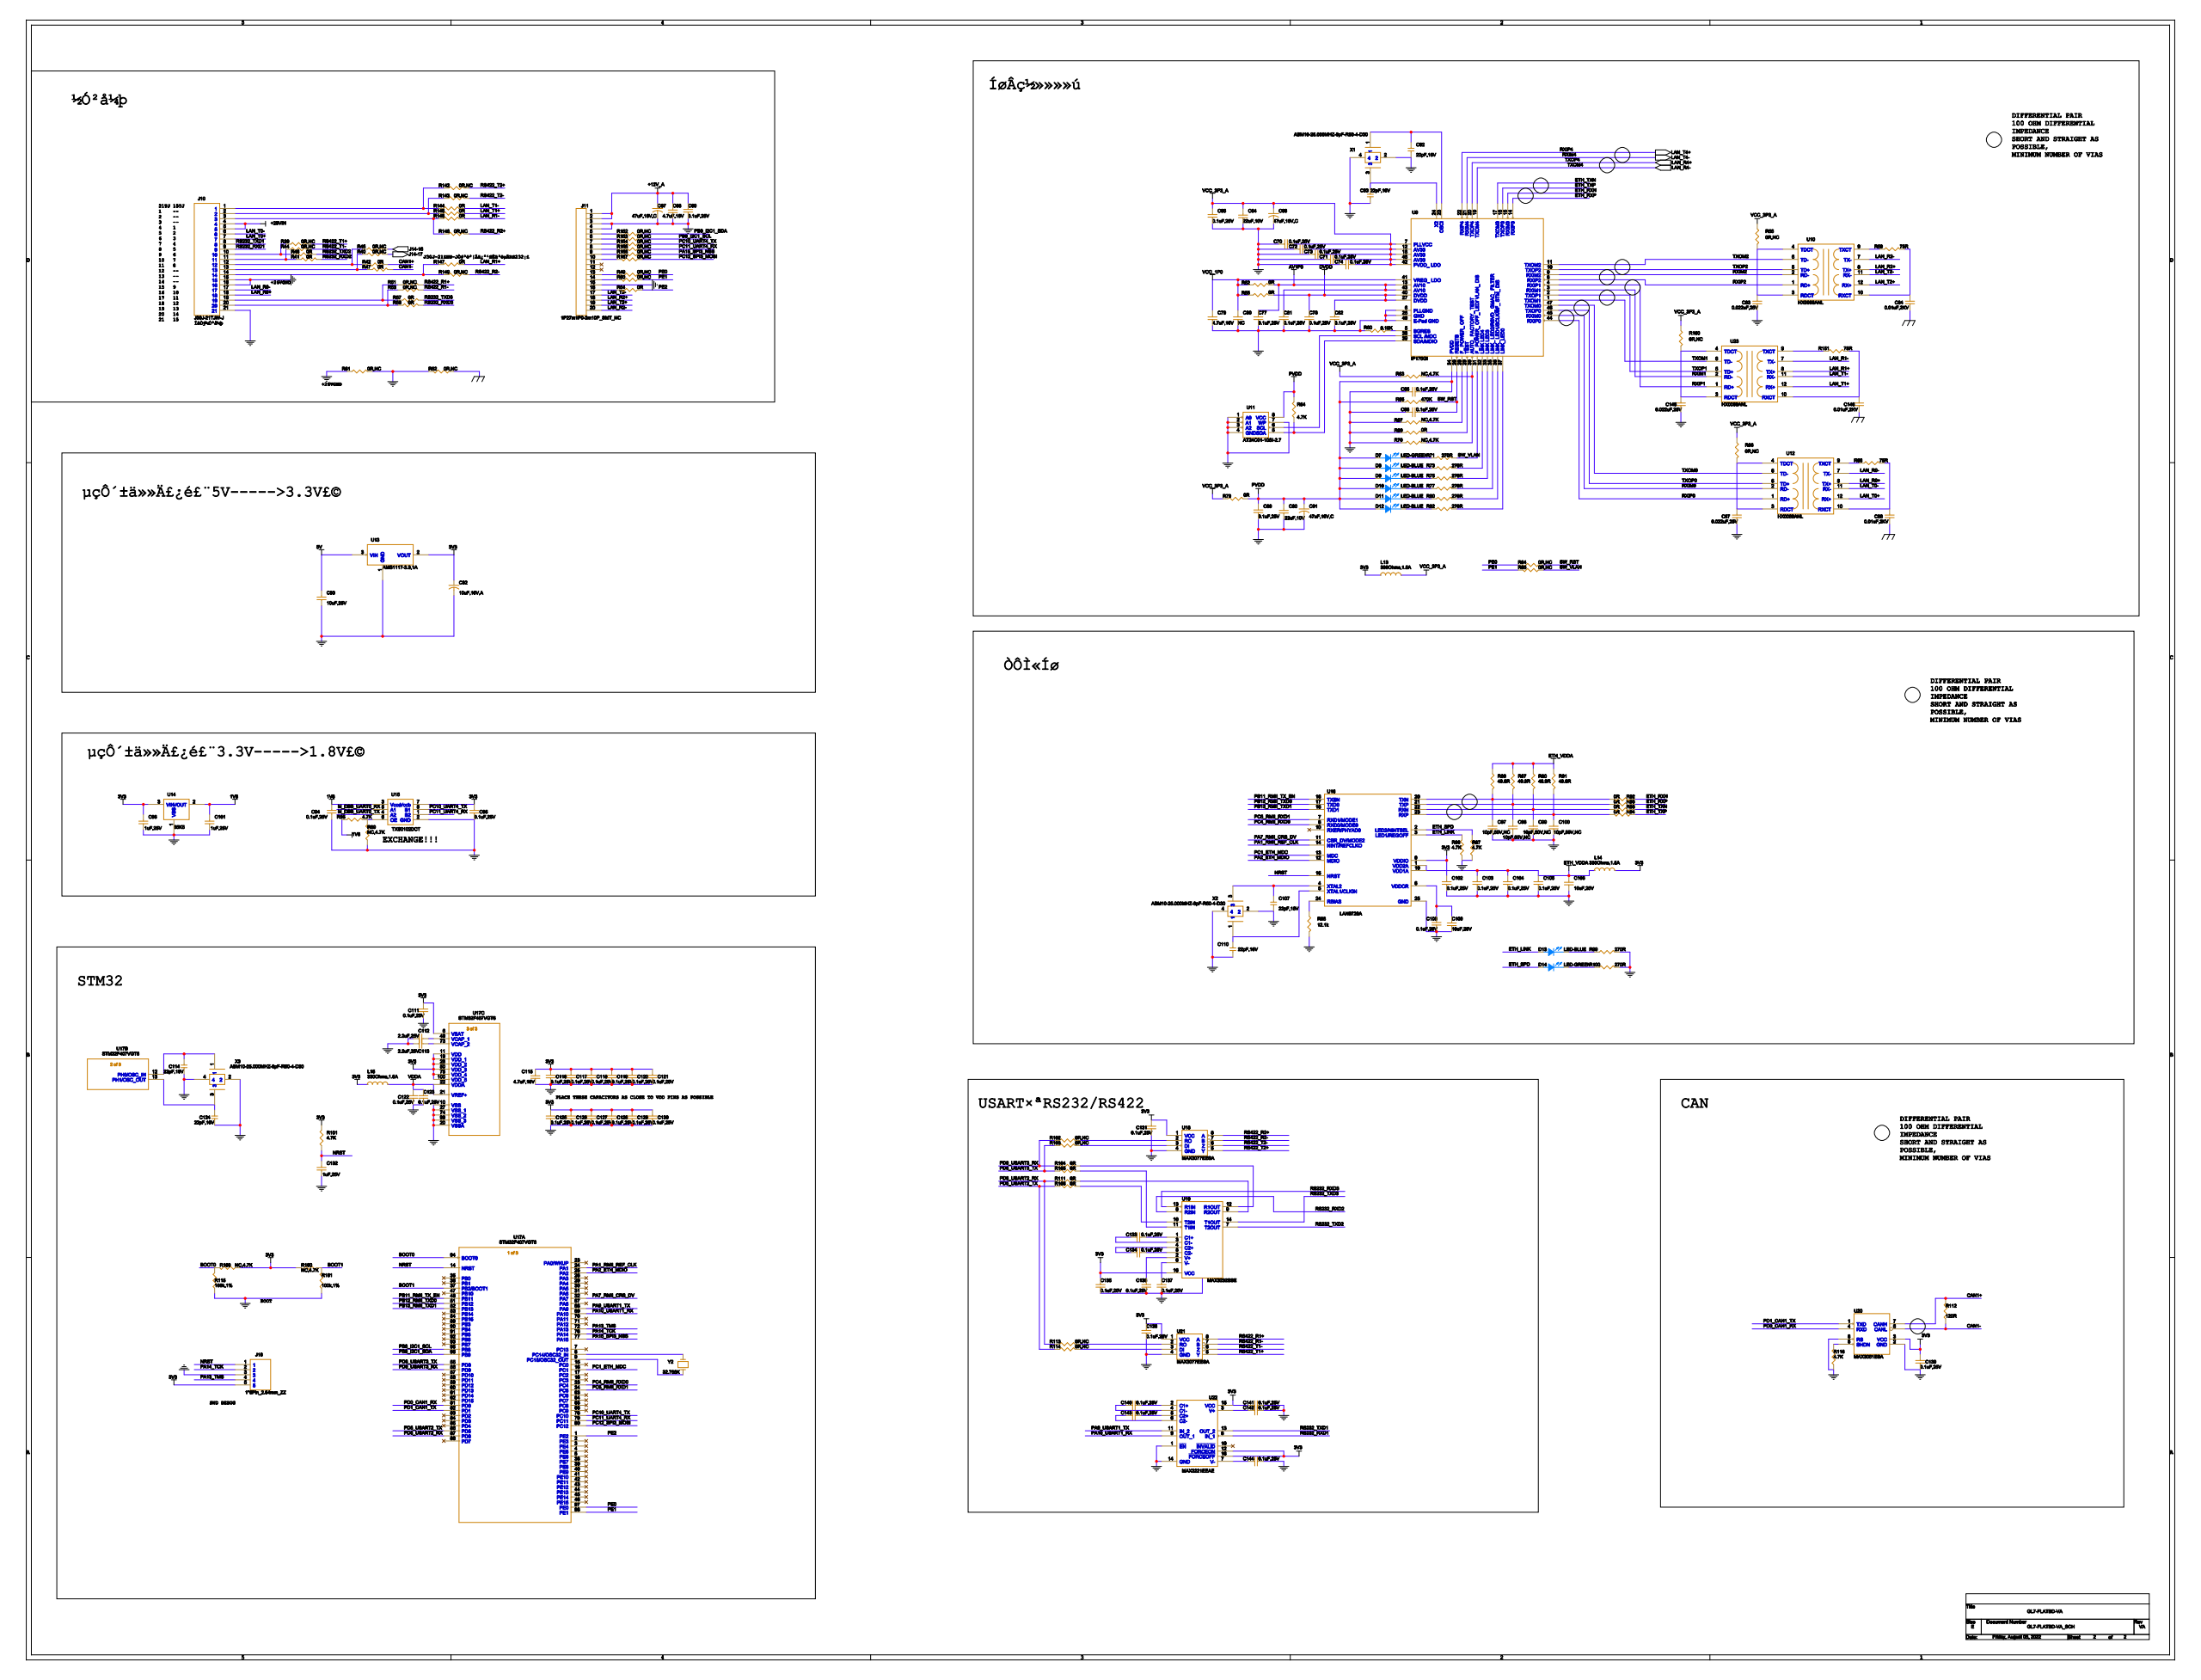Circuit board | Cadence Allegro | 338 parts | 273 nets | one sheet of the schematic
Parts on this sheet (reference | value | footprint):
C62 | 22pF,16V | 0402C
C63 | 22pF,16V | 0402C
C64 | 22uF,10V | 0603C
C65 | 0.1uF,25V | 0201C
C66 | 47uF,16V,C | CA45C
C67 | 47uF,16V,C | CA45C
C68 | 4.7uF,16V | 0603C
C69 | 0.1uF,25V | 0201C
C70 | 0.1uF,25V | 0201C
C71 | 0.1uF,25V | 0201C
C72 | 0.1uF,25V | 0201C
C73 | 0.1uF,25V | 0201C
C74 | 0.1uF,25V | 0201C
C77 | 0.1uF,25V | 0201C
C78 | 0.1uF,25V | 0201C
C79 | 4.7uF,16V | 0603C
C80 | NC | 0402C
C81 | 0.1uF,25V | 0201C
C82 | 0.1uF,25V | 0201C
C83 | 0.022uF,25V | 0402C
C84 | 0.01uF,2KV | 1812C
C85 | 0.1uF,25V | 0201C
C86 | 0.1uF,25V | 0201C
C87 | 0.022uF,25V | 0402C
C88 | 0.01uF,2KV | 1812C
C89 | 0.1uF,25V | 0201C
C90 | 22uF,10V | 0603C
C91 | 47uF,16V,C | CA45C
C92 | 10uF,16V,A | CA45A
C93 | 10uF,25V | 1206C
C94 | 0.1uF,25V | 0201C
C95 | 0.1uF,25V | 0201C
C96 | 1uF,25V | 0402C
C97 | NC | 0402C
C98 | NC | 0402C
C99 | NC | 0402C
C100 | NC | 0402C
C101 | 1uF,25V | 0402C
C102 | 0.1uF,25V | 0201C
C103 | 0.1uF,25V | 0201C
C104 | 0.1uF,25V | 0201C
C105 | 0.1uF,25V | 0201C
C106 | 10uF,25V | 1206C
C107 | 22pF,16V | 0402C
C108 | 0.1uF,25V | 0201C
C109 | 10uF,25V | 1206C
C110 | 22pF,16V | 0402C
C111 | 0.1uF,25V | 0201C
C112 | 2.2uF,25V | 0603C
C114 | 22pF,16V | 0402C
C115 | 4.7uF,16V | 0603C
C116 | 0.1uF,25V | 0201C
C117 | 0.1uF,25V | 0201C
C118 | 0.1uF,25V | 0201C
C119 | 0.1uF,25V | 0201C
C120 | 0.1uF,25V | 0201C
C121 | 0.1uF,25V | 0201C
C122 | 0.1uF,25V | 0201C
C123 | 0.1uF,25V | 0201C
C124 | 22pF,16V | 0402C
C125 | 0.1uF,25V | 0201C
C126 | 0.1uF,25V | 0201C
C127 | 0.1uF,25V | 0201C
C128 | 0.1uF,25V | 0201C
C129 | 0.1uF,25V | 0201C
C130 | 0.1uF,25V | 0201C
C131 | 0.1uF,25V | 0201C
C132 | 1uF,25V | 0402C
C133 | 0.1uF,25V | 0201C
C134 | 0.1uF,25V | 0201C
C135 | 0.1uF,25V | 0201C
C136 | 0.1uF,25V | 0201C
C137 | 0.1uF,25V | 0201C
C138 | 0.1uF,25V | 0201C
C139 | 0.1uF,25V | 0201C
C140 | 0.1uF,25V | 0201C
C141 | 0.1uF,25V | 0201C
C142 | 0.1uF,25V | 0201C
C143 | 0.1uF,25V | 0201C
C144 | 0.1uF,25V | 0201C
C145 | 0.022uF,25V | 0402C
C146 | 0.01uF,2KV | 1812C
D7 | LED-GREEN | 0603L
D8 | LED-BLUE | 0603L
D9 | LED-BLUE | 0603L
D10 | LED-BLUE | 0603L
D11 | LED-BLUE | 0603L
D12 | LED-BLUE | 0603L
D13 | LED-BLUE | 0603L
D14 | LED-GREEN | 0603L
J10 | J30J-21TJW-J | J30J-21TJW-J
J11 | 1P27m1P0-2m10P_SMT_NC | 1P27-2-10-L-SMT
J16 | 1*5Pin_2.54mm_ZZ | SIP-5-2R5
L13 | 330Ohms,1.5A | 0805L
L14 | 1.5A,330Ohms | 0805L
L15 | 1.5A,330Ohms | 0805L
R39 | 0R,NC | 0402R
R40 | 0R,NC | 0402R
R41 | 0R | 0402R
R42 | 0R | 0402R
R44 | 0R,NC | 0402R
R45 | 0R,NC | 0402R
R46 | 0R | 0402R
R47 | 0R | 0402R
R49 | 0R,NC | 0402R
R50 | 0R,NC | 0402R
R51 | 0R,NC | 0402R
R52 | 0R | 0402R
R53 | 0R,NC | 0402R
R54 | 0R | 0402R
R55 | 0R | 0402R
R56 | 0R,NC | 0402R
R57 | 0R | 0402R
R58 | 0R | 0402R
R59 | 75R | 0402R
R60 | 6.19K | 0603R
R61 | 0R,NC | 0805R
R62 | 0R,NC | 0805R
R63 | NC,4.7K | 0402R
R64 | 4.7K | 0402R
R65 | 470K | 0402R
R66 | 0R,NC | 0402R
R67 | NC,4.7K | 0402R
R68 | 75R | 0402R
R69 | 0R | 0402R
R70 | NC,4.7K | 0402R
R71 | 270R | 0402R
R73 | 270R | 0402R
R75 | 270R | 0402R
R77 | 270R | 0402R
R79 | 0R | 0402R
R80 | 270R | 0402R
R82 | 270R | 0402R
R84 | 0R,NC | 0805R
R85 | 0R,NC | 0805R
R86 | 49.9R | 0402R
R87 | 49.9R | 0402R
R88 | 0R | 0402R
R89 | 4.7K,NC | 0402R
R90 | 49.9R | 0402R
R91 | 49.9R | 0402R
R92 | 0R | 0402R
R93 | 0R | 0402R
R94 | 0R | 0402R
R95 | 4.7K | 0402R
R96 | 4.7K | 0402R
R97 | 4.7K | 0402R
R98 | 12K | 0402R
R99 | 270R | 0402R
R100 | 270R | 0402R
R101 | 4.7K | 0402R
R102 | 0R,NC | 0402R
R103 | 0R,NC | 0402R
R104 | 0R | 0402R
R105 | 0R | 0402R
R106 | 0R | 0402R
R111 | 0R | 0402R
R112 | 120R | 0805R
R113 | 0R,NC | 0402R
R114 | 0R,NC | 0402R
R115 | 100k | 0402R
R116 | 4.7K | 0402R
R142 | 0R,NC | 0402R
R143 | 0R,NC | 0402R
R144 | 0R | 0402R
R145 | 0R | 0402R
R146 | 0R | 0402R
R147 | 0R | 0402R
R148 | 0R,NC | 0402R
R149 | 0R,NC | 0402R
R150 | 0R,NC | 0402R
R151 | 75R | 0402R
R152 | 0R,NC | 0402R
R153 | 0R,NC | 0402R
R154 | 0R,NC | 0402R
R155 | 0R,NC | 0402R
R156 | 0R,NC | 0402R
R157 | 0R,NC | 0402R
R159 | 4.7K,NC | 0402R
R160 | 4.7K,NC | 0402R
R161 | 100k | 0402R
U9 | IP175GI | QFN_48
U10 | HX0068ANL | HX0068ANL
U11 | AT24C01-10SI-2.7 | SOIC8_300_206
U12 | HX0068ANL | HX0068ANL
U13 | AMS1117-3.3,1A | TO252AA
U14 | 65K5 | SOT23-28X44
U15 | TXS0102DCT | SSOP8-TXS0102DCT
U16 | LAN8720A | QFN24
U17 | STM32F407VGT6 | LQFP100-14X14MM
U18 | MAX3077EESA | SO8-25X75
U19 | MAX3232ESE | SOIC16
U20 | MAX3051ESA | SO8-25X75
U21 | MAX3077EESA | SO8-25X75
U22 | MAX3221EEAE | SSOP16
U23 | HX0068ANL | HX0068ANL
X1 | ABM10-25.000MHZ-8pF-R50-4-D30 | ABM10-2_5X2_0-0_55
X2 | ABM10-25.000MHZ-8pF-R50-4-D30 | ABM10-2_5X2_0-0_55
X3 | ABM10-25.000MHZ-8pF-R50-4-D30 | ABM10-2_5X2_0-0_55
Y2 | 32.768K | ABS06
Nets of these parts (net: part-pin ...):
+26VGND: R61-1 J10-15 J10-16
GND: C62-2 C63-2 C64-1 C65-2 C66-2 C67-2 C68-1 C69-2 C70-1 C71-1 C72-1 C73-1 C74-1 C77-1 C78-1 C79-1 C80-1 C81-1 C82-1 C83-2 C84-2 C85-2 C86-2 C87-2 C88-2 C89-2 C90-1 C91-2 C92-2 C93-1 C94-2 C95-2 C96-1 C97-1 C98-1 C99-1 C100-1 C101-1 C102-2 C103-2 C104-2 C105-2 C106-1 C107-2 C108-2 C109-1 C110-2 C111-2 C112-1 C114-2 C115-1 C116-2 C117-2 C118-2 C119-2 C120-2 C121-2 C122-2 C123-2 C124-2 C125-2 C126-2 C127-2 C128-2 C129-2 C130-2 C131-2 C132-1 C135-1 C136-1 C137-1 C138-1 C139-2 C141-1 C142-1 C144-1 C145-2 C146-2 J11-3 J11-4 J11-15 J16-3 R60-2 R61-2 R62-1 R62-2 R67-1 R69-1 R70-1 R89-1 R96-1 R97-1 R98-2 R99-2 R100-2 R115-1 R116-1 R161-1 U11-1 U11-2 U11-3 U11-4 U11-7 U13-1 U14-1 U15-2 U18-4 U19-15 U20-2 U20-8 U21-4 U22-1 U22-14 X1-2 X1-4 X2-2 X2-4 X3-2 X3-4 J10-21 U9-6 U9-25 U9-49 U16-25 U17-10 U17-20 U17-27 U17-74 U17-99
N17044993: C133-2 U19-1
N17045014: C133-1 U19-3
N17045028: C134-1 U19-4
N17045034: C134-2 U19-5
RS232_RXD3: R58-2 U19-13
N17045078: R104-2 U19-12
RS232_RXD2: R41-2 U19-8
N17045090: R111-2 U19-9
N17045064: R105-2 U19-11
RS232_TXD3: R57-2 U19-14
N17045084: R106-2 U19-10
RS232_TXD2: R46-2 U19-7
N17045046: C136-2 U19-2
N17045042: C137-2 U19-6
3V3: C92-1 C95-1 C96-2 C102-1 C111-1 C115-2 C116-1 C117-1 C118-1 C119-1 C120-1 C121-1 C125-1 C126-1 C127-1 C128-1 C129-1 C130-1 C131-1 C135-2 C138-2 C139-1 C141-2 J16-5 L13-2 L14-1 L15-2 R101-2 R159-1 R160-2 U13-2 U14-3 U15-7 U18-1 U19-16 U20-3 U21-1 U22-12 U22-15 U22-16 U16-9 U17-6 U17-11 U17-19 U17-28 U17-50 U17-75 U17-100
+12V_A: C67-1 C68-2 C69-1 J11-1 J11-2
5V: C93-2 U13-3
BOOT0: R115-2 R159-2 U17-94
BOOT1: R160-1 R161-2 U17-37
N17710352: C145-1 R150-2 U23-3 U23-4
N17694470: C83-1 R56-2 U10-3 U10-4
N17690042: C87-1 R66-2 U12-3 U12-4
VCC_1P0: C79-2 C80-2 R52-1 R55-1 U9-41
+26VIN: J10-4 J10-5
N17707313: R142-1 R144-1 J10-1
N17629569: R39-1 R46-1 J10-10
N17629581: R41-1 R44-1 J10-11
N17620450: R42-1 R45-1 J10-12
N17620485: R40-1 R47-1 J10-13
N17707523: R147-1 R149-1 J10-14
LAN_R0-: U12-7 J10-17
LAN_R0+: U12-8 J10-18
N17629552: R51-1 R57-1 J10-19
N17707328: R143-1 R145-1 J10-2
N17629572: R53-1 R58-1 J10-20
N17707373: R146-1 R148-1 J10-3
LAN_T0-: U12-11 J10-6
LAN_T0+: U12-12 J10-7
RS232_TXD1: U22-13 J10-8
RS232_RXD1: U22-8 J10-9
NRST: C132-2 J16-1 R101-1 U16-15 U17-14
PA14_TCK: J16-2 U17-76
PA13_TMS: J16-4 U17-72
N17048435: R98-1 U16-24
N17047452: D13-2 R99-1
N17047471: D14-2 R100-1
N17043700: D7-2 R71-1
SW_VLAN: R71-2 R85-1 U9-31
N17044896: D8-2 R73-1
N17044311: R73-2 U9-32
N17044898: D9-2 R75-1
N17044333: R75-2 U9-33
N17044902: D10-2 R77-1
N17044337: R77-2 U9-35
N17044904: D11-2 R80-1
N17044357: R80-2 U9-36
N17044906: D12-2 R82-1
N17044361: R82-2 U9-37
PB9_I2C1_SDA: R152-1 U17-96
N17729713: J11-5 R152-2
PB8_I2C1_SCL: R153-1 U17-95
N17729716: J11-6 R153-2
PC10_UART4_TX: R154-1 U15-8 U17-78
N17729719: J11-7 R154-2
PC11_UART4_RX: R155-1 U15-1 U17-79
N17729722: J11-8 R155-2
PA15_SPI3_NSS: R156-1 U17-77
N17729725: J11-9 R156-2
PC12_SPI3_MOSI: R157-1 U17-80
N17729728: J11-10 R157-2
PE0: R49-1 R84-2 U17-97
N17646911: J11-13 R49-2
PE1: R50-1 R85-2 U17-98
N17646914: J11-14 R50-2
VCC_3P3_A: C64-2 C65-1 C66-1 C70-2 C71-2 C72-2 C73-2 C74-2 L13-1 R56-1 R63-1 R66-1 R79-1 R150-1 U9-7 U9-12 U9-18 U9-42 U9-48
J14-16: R45-2
PD9_USART3_RX: R102-1 R104-1 U17-56
N17045208: R102-2 U18-2
PD8_USART3_TX: R103-1 R105-1 U17-55
N17045210: R103-2 U18-3
PD6_USART2_RX: R111-1 R113-1 U17-87
N17045561: R113-2 U21-2
PD5_USART2_TX: R106-1 R114-1 U17-86
N17045563: R114-2 U21-3
RS422_T2+: R142-2 U18-5
RS422_T2-: R143-2 U18-6
RS422_R2+: R148-2 U18-8
RS422_R2-: R149-2 U18-7
RS422_T1+: R39-2 U21-5
RS422_T1-: R44-2 U21-6
RS422_R1+: R51-2 U21-8
RS422_R1-: R53-2 U21-7
J14-17: R40-2
N17569056: R89-2 R95-2 U15-6
LAN_R4-: U9-19
LAN_R4+: U9-20
LAN_T4-: U9-21
LAN_T4+: U9-22
N17046201: R60-1 U9-5
SW_RST: C86-1 R65-2 R84-1 U9-26
ETH_VDDA: C103-1 C104-1 C105-1 C106-2 L14-2 R86-1 R87-1 R90-1 R91-1 U16-1 U16-19
N17045361: C97-2 R86-2 R92-1 U16-20
N17045365: C99-2 R88-1 R90-2 U16-22
N17045363: C98-2 R87-2 R93-1 U16-21
N17045367: C100-2 R91-2 R94-1 U16-23
M_DBB_UART0_RX: U15-5
M_DBB_UART0_TX: U15-4
1V8: C94-1 C101-2 R95-1 U14-2 U15-3
VDDA: C122-1 C123-1 L15-1 U17-21 U17-22
DVDD: C78-2 C82-2 R55-2 U9-27 U9-40
N17044214: C108-1 C109-2 U16-6
N17047971: C140-1 U22-2
N17047973: C140-2 U22-4
N17047979: C143-1 U22-5
N17047981: C143-2 U22-6
N17048080: C144-2 U22-7
N17048078: C142-2 U22-3
AV1P0: C77-2 C81-2 R52-2 U9-13 U9-43
PVDD: C85-1 C89-1 C90-2 C91-1 D7-1 D8-1 D9-1 D10-1 D11-1 D12-1 R64-2 R65-1 R79-2 U11-8 U9-34
N17045954: C107-1 X2-3 U16-4
N17046072: C62-1 X1-1 U9-23
N17044739: C114-1 X3-1 U17-12
N17045970: C110-1 X2-1 U16-5
N17044753: C124-1 X3-3 U17-13
N17046074: C63-1 X1-3 U9-24
N17046602: C112-2 U17-49
N17710358: C146-1 R151-2 U23-10
N17694476: C84-1 R59-2 U10-10
N17692703: C88-1 R68-2 U12-10
N17643248: J11-16 R54-2
LAN_T2-: J11-17 U10-11
LAN_R2+: J11-18 U10-8
LAN_T2+: J11-19 U10-12
LAN_R2-: J11-20 U10-7
CAN1-: R47-2 R112-1 U20-6
CAN1+: R42-2 R112-2 U20-7
N17710356: R151-1 U23-9
N17694474: R59-1 U10-9
N17692788: R68-1 U12-9
N17046670: R67-2 U9-28
N17046414: R63-2 R70-2 U9-30
PA1_RMII_REF_CLK: U16-14 U17-24
PA10_USART1_RX: U22-9 U17-69
PA2_ETH_MDIO: U16-12 U17-25
PA7_RMII_CRS_DV: U16-11 U17-32
PA9_USART1_TX: U22-11 U17-68
PB11_RMII_TX_EN: U16-16 U17-48
PB12_RMII_TXD0: U16-17 U17-51
PB13_RMII_TXD1: U16-18 U17-52
PC1_ETH_MDC: U16-13 U17-16
N17046188: Y2-2 U17-8
N17046190: Y2-1 U17-9
PC4_RMII_RXD0: U16-8 U17-33
PC5_RMII_RXD1: U16-7 U17-34
PD0_CAN1_RX: U20-4 U17-81
PD1_CAN1_TX: U20-1 U17-82
PE2: R54-1 U17-1
RXIP2: U10-1 U9-8
RXIM2: U10-2 U9-9
TXOP2: U10-5 U9-10
TXOM2: U10-6 U9-11
RXIP0: U12-1 U9-44
RXIM0: U12-2 U9-45
TXOP0: U12-5 U9-46
TXOM0: U12-6 U9-47
RXIP1: U23-1 U9-4
RXIM1: U23-2 U9-3
LAN_T1+: R145-2 U23-12
LAN_T1-: R144-2 U23-11
TXOP1: U23-5 U9-2
TXOM1: U23-6 U9-1
LAN_R1+: R147-2 U23-8
LAN_R1-: R146-2 U23-7
ETH_LINK: D13-1 R96-2 U16-3
ETH_SPD: D14-1 R97-2 U16-2
ETH_RXP: R93-2 U9-14
N17046915: R69-2 U9-29
ETH_RXN: R92-2 U9-15
ETH_TXN: R88-2 U9-17
ETH_TXP: R94-2 U9-16
N17048485: R116-2 U20-5
N17045022: R64-1 U11-5 U9-39
N17045016: U11-6 U9-38